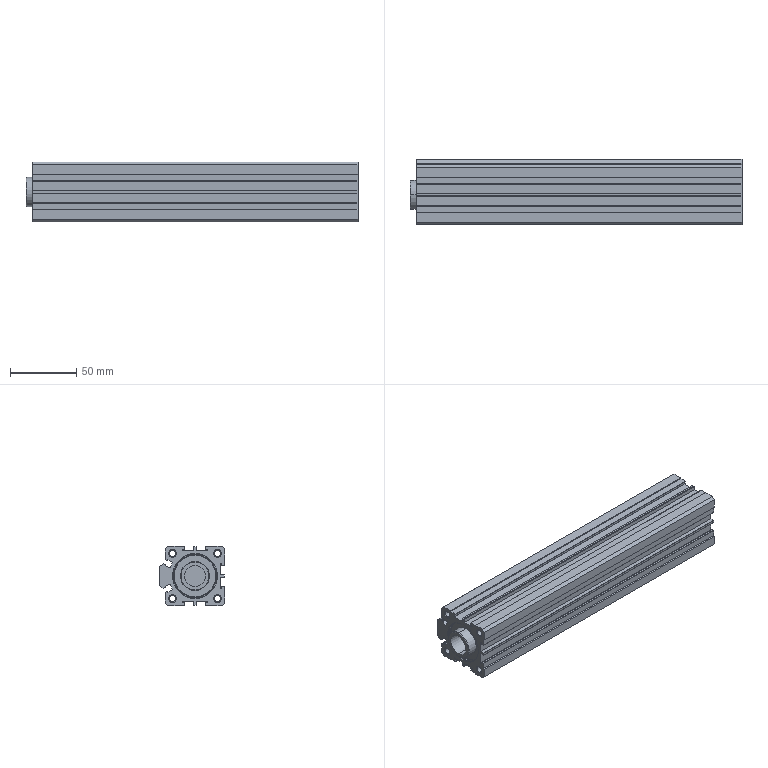Part | STEP file | 001-003-ACQS_32x200_B_P_b | 1 solid | 202 faces | box 250.5 x 49.5 x 45 mm | volume 256308 mm3 | plane 84 | cylinder 78 | cone 32 | torus 8 | commonest cylinder face diameters 0.4 x35 0.8 x10 4.917 x8 32 x8 22 x4 34 x4